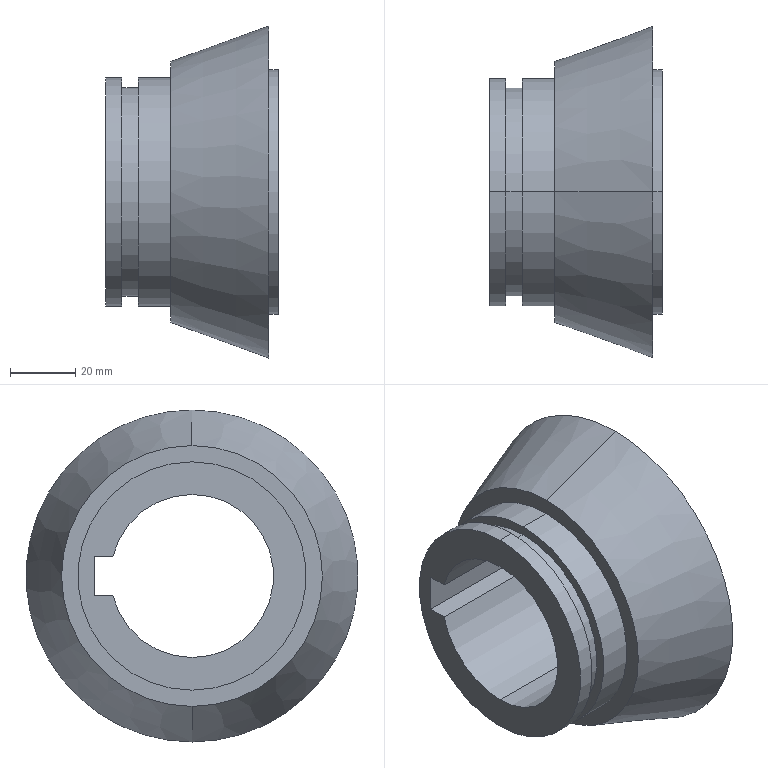Part | SolidWorks | features ICE 2, Revolution 1 | 1 solid | 25 faces | box 53 x 101.838 x 101.838 mm | volume 175302 mm3 | cylinder 13 | plane 10 | cone 2 | commonest cylinder face diameters 70 x4 50 x3 3 x2 64 x2 75 x2
STEP:
#1=CARTESIAN_POINT('',(43.,-32.5,1.5));
#2=VERTEX_POINT('',#1);
#3=CARTESIAN_POINT('',(43.,-32.5,-1.5));
#4=VERTEX_POINT('',#3);
#5=CARTESIAN_POINT('',(43.,-32.5,0.));
#6=DIRECTION('',(1.,0.,0.));
#7=DIRECTION('',(0.,0.,-1.));
#8=AXIS2_PLACEMENT_3D('',#5,#6,#7);
#9=CIRCLE('',#8,1.5);
#10=EDGE_CURVE('',#2,#4,#9,.T.);
#11=ORIENTED_EDGE('',*,*,#10,.F.);
#12=CARTESIAN_POINT('',(53.,-32.5,1.5));
#13=VERTEX_POINT('',#12);
#14=CARTESIAN_POINT('',(43.,-32.5,1.5));
#15=DIRECTION('',(1.,0.,0.));
#16=VECTOR('',#15,1000.);
#17=LINE('',#14,#16);
#18=EDGE_CURVE('',#2,#13,#17,.T.);
#19=ORIENTED_EDGE('',*,*,#18,.T.);
#20=CARTESIAN_POINT('',(53.,-32.5,-1.5));
#21=VERTEX_POINT('',#20);
#22=CARTESIAN_POINT('',(53.,-32.5,0.));
#23=DIRECTION('',(1.,0.,0.));
#24=DIRECTION('',(0.,0.,-1.));
#25=AXIS2_PLACEMENT_3D('',#22,#23,#24);
#26=CIRCLE('',#25,1.5);
#27=EDGE_CURVE('',#13,#21,#26,.T.);
#28=ORIENTED_EDGE('',*,*,#27,.T.);
#29=CARTESIAN_POINT('',(43.,-32.5,-1.5));
#30=DIRECTION('',(1.,0.,0.));
#31=VECTOR('',#30,1000.);
#32=LINE('',#29,#31);
#33=EDGE_CURVE('',#4,#21,#32,.T.);
#34=ORIENTED_EDGE('',*,*,#33,.F.);
#35=EDGE_LOOP('',(#11,#19,#28,#34));
#36=FACE_OUTER_BOUND('',#35,.T.);
#37=CARTESIAN_POINT('',(43.,-32.5,0.));
#38=DIRECTION('',(1.,0.,0.));
#39=DIRECTION('',(0.,0.,-1.));
#40=AXIS2_PLACEMENT_3D('',#37,#38,#39);
#41=CYLINDRICAL_SURFACE('',#40,1.5);
#42=ADVANCED_FACE('',(#36),#41,.F.);
#43=CARTESIAN_POINT('',(53.,0.,37.5));
#44=VERTEX_POINT('',#43);
#45=CARTESIAN_POINT('',(53.,0.,-37.5));
#46=VERTEX_POINT('',#45);
#47=CARTESIAN_POINT('',(53.,0.,0.));
#48=DIRECTION('',(-1.,0.,0.));
#49=DIRECTION('',(0.,0.,1.));
#50=AXIS2_PLACEMENT_3D('',#47,#48,#49);
#51=CIRCLE('',#50,37.5);
#52=EDGE_CURVE('',#44,#46,#51,.T.);
#53=ORIENTED_EDGE('',*,*,#52,.T.);
#54=CARTESIAN_POINT('',(50.,0.,-37.5));
#55=VERTEX_POINT('',#54);
#56=CARTESIAN_POINT('',(0.,0.,-37.5));
#57=DIRECTION('',(-1.,0.,0.));
#58=VECTOR('',#57,1000.);
#59=LINE('',#56,#58);
#60=EDGE_CURVE('',#46,#55,#59,.T.);
#61=ORIENTED_EDGE('',*,*,#60,.T.);
#62=CARTESIAN_POINT('',(50.,0.,37.5));
#63=VERTEX_POINT('',#62);
#64=CARTESIAN_POINT('',(50.,0.,0.));
#65=DIRECTION('',(-1.,0.,0.));
#66=DIRECTION('',(0.,0.,1.));
#67=AXIS2_PLACEMENT_3D('',#64,#65,#66);
#68=CIRCLE('',#67,37.5);
#69=EDGE_CURVE('',#63,#55,#68,.T.);
#70=ORIENTED_EDGE('',*,*,#69,.F.);
#71=CARTESIAN_POINT('',(0.,0.,37.5));
#72=DIRECTION('',(-1.,0.,0.));
#73=VECTOR('',#72,1000.);
#74=LINE('',#71,#73);
#75=EDGE_CURVE('',#44,#63,#74,.T.);
#76=ORIENTED_EDGE('',*,*,#75,.F.);
#77=EDGE_LOOP('',(#53,#61,#70,#76));
#78=FACE_OUTER_BOUND('',#77,.T.);
#79=CARTESIAN_POINT('',(0.,0.,0.));
#80=DIRECTION('',(-1.,0.,0.));
#81=DIRECTION('',(0.,0.,1.));
#82=AXIS2_PLACEMENT_3D('',#79,#80,#81);
#83=CYLINDRICAL_SURFACE('',#82,37.5);
#84=ADVANCED_FACE('',(#78),#83,.T.);
#85=CARTESIAN_POINT('',(20.,0.,40.));
#86=VERTEX_POINT('',#85);
#87=CARTESIAN_POINT('',(20.,0.,-40.));
#88=VERTEX_POINT('',#87);
#89=CARTESIAN_POINT('',(20.,0.,0.));
#90=DIRECTION('',(-1.,0.,0.));
#91=DIRECTION('',(0.,0.,1.));
#92=AXIS2_PLACEMENT_3D('',#89,#90,#91);
#93=CIRCLE('',#92,40.);
#94=EDGE_CURVE('',#86,#88,#93,.T.);
#95=ORIENTED_EDGE('',*,*,#94,.F.);
#96=CARTESIAN_POINT('',(50.,0.,50.919));
#97=VERTEX_POINT('',#96);
#98=CARTESIAN_POINT('',(50.,0.,50.919));
#99=DIRECTION('',(0.9397,0.,0.342));
#100=VECTOR('',#99,1000.);
#101=LINE('',#98,#100);
#102=EDGE_CURVE('',#86,#97,#101,.T.);
#103=ORIENTED_EDGE('',*,*,#102,.T.);
#104=CARTESIAN_POINT('',(50.,0.,-50.919));
#105=VERTEX_POINT('',#104);
#106=CARTESIAN_POINT('',(50.,0.,0.));
#107=DIRECTION('',(-1.,0.,0.));
#108=DIRECTION('',(0.,0.,1.));
#109=AXIS2_PLACEMENT_3D('',#106,#107,#108);
#110=CIRCLE('',#109,50.919);
#111=EDGE_CURVE('',#97,#105,#110,.T.);
#112=ORIENTED_EDGE('',*,*,#111,.T.);
#113=CARTESIAN_POINT('',(50.,0.,-50.919));
#114=DIRECTION('',(0.9397,0.,-0.342));
#115=VECTOR('',#114,1000.);
#116=LINE('',#113,#115);
#117=EDGE_CURVE('',#88,#105,#116,.T.);
#118=ORIENTED_EDGE('',*,*,#117,.F.);
#119=EDGE_LOOP('',(#95,#103,#112,#118));
#120=FACE_OUTER_BOUND('',#119,.T.);
#121=CARTESIAN_POINT('',(50.,0.,0.));
#122=DIRECTION('',(1.,0.,0.));
#123=DIRECTION('',(0.,0.,-1.));
#124=AXIS2_PLACEMENT_3D('',#121,#122,#123);
#125=CONICAL_SURFACE('',#124,50.919,0.3491);
#126=ADVANCED_FACE('',(#120),#125,.T.);
#127=CARTESIAN_POINT('',(20.,0.,35.));
#128=VERTEX_POINT('',#127);
#129=CARTESIAN_POINT('',(20.,0.,-35.));
#130=VERTEX_POINT('',#129);
#131=CARTESIAN_POINT('',(20.,0.,0.));
#132=DIRECTION('',(-1.,0.,0.));
#133=DIRECTION('',(0.,0.,1.));
#134=AXIS2_PLACEMENT_3D('',#131,#132,#133);
#135=CIRCLE('',#134,35.);
#136=EDGE_CURVE('',#128,#130,#135,.T.);
#137=ORIENTED_EDGE('',*,*,#136,.T.);
#138=CARTESIAN_POINT('',(10.,0.,-35.));
#139=VERTEX_POINT('',#138);
#140=CARTESIAN_POINT('',(0.,0.,-35.));
#141=DIRECTION('',(-1.,0.,0.));
#142=VECTOR('',#141,1000.);
#143=LINE('',#140,#142);
#144=EDGE_CURVE('',#130,#139,#143,.T.);
#145=ORIENTED_EDGE('',*,*,#144,.T.);
#146=CARTESIAN_POINT('',(10.,0.,35.));
#147=VERTEX_POINT('',#146);
#148=CARTESIAN_POINT('',(10.,0.,0.));
#149=DIRECTION('',(-1.,0.,0.));
#150=DIRECTION('',(0.,0.,1.));
#151=AXIS2_PLACEMENT_3D('',#148,#149,#150);
#152=CIRCLE('',#151,35.);
#153=EDGE_CURVE('',#147,#139,#152,.T.);
#154=ORIENTED_EDGE('',*,*,#153,.F.);
#155=CARTESIAN_POINT('',(0.,0.,35.));
#156=DIRECTION('',(-1.,0.,0.));
#157=VECTOR('',#156,1000.);
#158=LINE('',#155,#157);
#159=EDGE_CURVE('',#128,#147,#158,.T.);
#160=ORIENTED_EDGE('',*,*,#159,.F.);
#161=EDGE_LOOP('',(#137,#145,#154,#160));
#162=FACE_OUTER_BOUND('',#161,.T.);
#163=CARTESIAN_POINT('',(0.,0.,0.));
#164=DIRECTION('',(-1.,0.,0.));
#165=DIRECTION('',(0.,0.,1.));
#166=AXIS2_PLACEMENT_3D('',#163,#164,#165);
#167=CYLINDRICAL_SURFACE('',#166,35.);
#168=ADVANCED_FACE('',(#162),#167,.T.);
#169=CARTESIAN_POINT('',(10.,0.,32.));
#170=VERTEX_POINT('',#169);
#171=CARTESIAN_POINT('',(10.,0.,-32.));
#172=VERTEX_POINT('',#171);
#173=CARTESIAN_POINT('',(10.,0.,0.));
#174=DIRECTION('',(-1.,0.,0.));
#175=DIRECTION('',(0.,0.,1.));
#176=AXIS2_PLACEMENT_3D('',#173,#174,#175);
#177=CIRCLE('',#176,32.);
#178=EDGE_CURVE('',#170,#172,#177,.T.);
#179=ORIENTED_EDGE('',*,*,#178,.T.);
#180=CARTESIAN_POINT('',(5.,0.,-32.));
#181=VERTEX_POINT('',#180);
#182=CARTESIAN_POINT('',(0.,0.,-32.));
#183=DIRECTION('',(-1.,0.,0.));
#184=VECTOR('',#183,1000.);
#185=LINE('',#182,#184);
#186=EDGE_CURVE('',#172,#181,#185,.T.);
#187=ORIENTED_EDGE('',*,*,#186,.T.);
#188=CARTESIAN_POINT('',(5.,0.,32.));
#189=VERTEX_POINT('',#188);
#190=CARTESIAN_POINT('',(5.,0.,0.));
#191=DIRECTION('',(-1.,0.,0.));
#192=DIRECTION('',(0.,0.,1.));
#193=AXIS2_PLACEMENT_3D('',#190,#191,#192);
#194=CIRCLE('',#193,32.);
#195=EDGE_CURVE('',#189,#181,#194,.T.);
#196=ORIENTED_EDGE('',*,*,#195,.F.);
#197=CARTESIAN_POINT('',(0.,0.,32.));
#198=DIRECTION('',(-1.,0.,0.));
#199=VECTOR('',#198,1000.);
#200=LINE('',#197,#199);
#201=EDGE_CURVE('',#170,#189,#200,.T.);
#202=ORIENTED_EDGE('',*,*,#201,.F.);
#203=EDGE_LOOP('',(#179,#187,#196,#202));
#204=FACE_OUTER_BOUND('',#203,.T.);
#205=CARTESIAN_POINT('',(0.,0.,0.));
#206=DIRECTION('',(-1.,0.,0.));
#207=DIRECTION('',(0.,0.,1.));
#208=AXIS2_PLACEMENT_3D('',#205,#206,#207);
#209=CYLINDRICAL_SURFACE('',#208,32.);
#210=ADVANCED_FACE('',(#204),#209,.T.);
#211=CARTESIAN_POINT('',(5.,0.,35.));
#212=VERTEX_POINT('',#211);
#213=CARTESIAN_POINT('',(5.,0.,-35.));
#214=VERTEX_POINT('',#213);
#215=CARTESIAN_POINT('',(5.,0.,0.));
#216=DIRECTION('',(-1.,0.,0.));
#217=DIRECTION('',(0.,0.,1.));
#218=AXIS2_PLACEMENT_3D('',#215,#216,#217);
#219=CIRCLE('',#218,35.);
#220=EDGE_CURVE('',#212,#214,#219,.T.);
#221=ORIENTED_EDGE('',*,*,#220,.T.);
#222=CARTESIAN_POINT('',(0.,0.,-35.));
#223=VERTEX_POINT('',#222);
#224=CARTESIAN_POINT('',(0.,0.,-35.));
#225=DIRECTION('',(-1.,0.,0.));
#226=VECTOR('',#225,1000.);
#227=LINE('',#224,#226);
#228=EDGE_CURVE('',#214,#223,#227,.T.);
#229=ORIENTED_EDGE('',*,*,#228,.T.);
#230=CARTESIAN_POINT('',(0.,0.,35.));
#231=VERTEX_POINT('',#230);
#232=CARTESIAN_POINT('',(0.,0.,0.));
#233=DIRECTION('',(-1.,0.,0.));
#234=DIRECTION('',(0.,0.,1.));
#235=AXIS2_PLACEMENT_3D('',#232,#233,#234);
#236=CIRCLE('',#235,35.);
#237=EDGE_CURVE('',#231,#223,#236,.T.);
#238=ORIENTED_EDGE('',*,*,#237,.F.);
#239=CARTESIAN_POINT('',(0.,0.,35.));
#240=DIRECTION('',(-1.,0.,0.));
#241=VECTOR('',#240,1000.);
#242=LINE('',#239,#241);
#243=EDGE_CURVE('',#212,#231,#242,.T.);
#244=ORIENTED_EDGE('',*,*,#243,.F.);
#245=EDGE_LOOP('',(#221,#229,#238,#244));
#246=FACE_OUTER_BOUND('',#245,.T.);
#247=CARTESIAN_POINT('',(0.,0.,0.));
#248=DIRECTION('',(-1.,0.,0.));
#249=DIRECTION('',(0.,0.,1.));
#250=AXIS2_PLACEMENT_3D('',#247,#248,#249);
#251=CYLINDRICAL_SURFACE('',#250,35.);
#252=ADVANCED_FACE('',(#246),#251,.T.);
#253=CARTESIAN_POINT('',(53.,0.,-25.));
#254=VERTEX_POINT('',#253);
#255=CARTESIAN_POINT('',(53.,0.,25.));
#256=VERTEX_POINT('',#255);
#257=CARTESIAN_POINT('',(53.,0.,0.));
#258=DIRECTION('',(-1.,0.,0.));
#259=DIRECTION('',(0.,0.,1.));
#260=AXIS2_PLACEMENT_3D('',#257,#258,#259);
#261=CIRCLE('',#260,25.);
#262=EDGE_CURVE('',#254,#256,#261,.T.);
#263=ORIENTED_EDGE('',*,*,#262,.F.);
#264=CARTESIAN_POINT('',(0.,0.,-25.));
#265=VERTEX_POINT('',#264);
#266=CARTESIAN_POINT('',(0.,0.,-25.));
#267=DIRECTION('',(-1.,0.,0.));
#268=VECTOR('',#267,1000.);
#269=LINE('',#266,#268);
#270=EDGE_CURVE('',#254,#265,#269,.T.);
#271=ORIENTED_EDGE('',*,*,#270,.T.);
#272=CARTESIAN_POINT('',(0.,0.,25.));
#273=VERTEX_POINT('',#272);
#274=CARTESIAN_POINT('',(0.,0.,0.));
#275=DIRECTION('',(-1.,0.,0.));
#276=DIRECTION('',(0.,0.,1.));
#277=AXIS2_PLACEMENT_3D('',#274,#275,#276);
#278=CIRCLE('',#277,25.);
#279=EDGE_CURVE('',#265,#273,#278,.T.);
#280=ORIENTED_EDGE('',*,*,#279,.T.);
#281=CARTESIAN_POINT('',(0.,0.,25.));
#282=DIRECTION('',(-1.,0.,0.));
#283=VECTOR('',#282,1000.);
#284=LINE('',#281,#283);
#285=EDGE_CURVE('',#256,#273,#284,.T.);
#286=ORIENTED_EDGE('',*,*,#285,.F.);
#287=EDGE_LOOP('',(#263,#271,#280,#286));
#288=FACE_OUTER_BOUND('',#287,.T.);
#289=CARTESIAN_POINT('',(0.,0.,0.));
#290=DIRECTION('',(-1.,0.,0.));
#291=DIRECTION('',(0.,0.,1.));
#292=AXIS2_PLACEMENT_3D('',#289,#290,#291);
#293=CYLINDRICAL_SURFACE('',#292,25.);
#294=ADVANCED_FACE('',(#288),#293,.F.);
#295=CARTESIAN_POINT('',(53.,24.269,6.));
#296=VERTEX_POINT('',#295);
#297=CARTESIAN_POINT('',(53.,0.,0.));
#298=DIRECTION('',(-1.,0.,0.));
#299=DIRECTION('',(0.,0.,1.));
#300=AXIS2_PLACEMENT_3D('',#297,#298,#299);
#301=CIRCLE('',#300,25.);
#302=EDGE_CURVE('',#256,#296,#301,.T.);
#303=ORIENTED_EDGE('',*,*,#302,.F.);
#304=ORIENTED_EDGE('',*,*,#285,.T.);
#305=CARTESIAN_POINT('',(0.,24.269,6.));
#306=VERTEX_POINT('',#305);
#307=CARTESIAN_POINT('',(0.,0.,0.));
#308=DIRECTION('',(-1.,0.,0.));
#309=DIRECTION('',(0.,0.,1.));
#310=AXIS2_PLACEMENT_3D('',#307,#308,#309);
#311=CIRCLE('',#310,25.);
#312=EDGE_CURVE('',#273,#306,#311,.T.);
#313=ORIENTED_EDGE('',*,*,#312,.T.);
#314=CARTESIAN_POINT('',(0.,24.269,6.));
#315=DIRECTION('',(1.,0.,0.));
#316=VECTOR('',#315,1000.);
#317=LINE('',#314,#316);
#318=EDGE_CURVE('',#306,#296,#317,.T.);
#319=ORIENTED_EDGE('',*,*,#318,.T.);
#320=EDGE_LOOP('',(#303,#304,#313,#319));
#321=FACE_OUTER_BOUND('',#320,.T.);
#322=CARTESIAN_POINT('',(0.,0.,0.));
#323=DIRECTION('',(-1.,0.,0.));
#324=DIRECTION('',(0.,0.,1.));
#325=AXIS2_PLACEMENT_3D('',#322,#323,#324);
#326=CYLINDRICAL_SURFACE('',#325,25.);
#327=ADVANCED_FACE('',(#321),#326,.F.);
#328=ORIENTED_EDGE('',*,*,#270,.F.);
#329=CARTESIAN_POINT('',(53.,24.269,-6.));
#330=VERTEX_POINT('',#329);
#331=CARTESIAN_POINT('',(53.,0.,0.));
#332=DIRECTION('',(-1.,0.,0.));
#333=DIRECTION('',(0.,0.,1.));
#334=AXIS2_PLACEMENT_3D('',#331,#332,#333);
#335=CIRCLE('',#334,25.);
#336=EDGE_CURVE('',#330,#254,#335,.T.);
#337=ORIENTED_EDGE('',*,*,#336,.F.);
#338=CARTESIAN_POINT('',(0.,24.269,-6.));
#339=VERTEX_POINT('',#338);
#340=CARTESIAN_POINT('',(0.,24.269,-6.));
#341=DIRECTION('',(-1.,0.,0.));
#342=VECTOR('',#341,1000.);
#343=LINE('',#340,#342);
#344=EDGE_CURVE('',#330,#339,#343,.T.);
#345=ORIENTED_EDGE('',*,*,#344,.T.);
#346=CARTESIAN_POINT('',(0.,0.,0.));
#347=DIRECTION('',(-1.,0.,0.));
#348=DIRECTION('',(0.,0.,1.));
#349=AXIS2_PLACEMENT_3D('',#346,#347,#348);
#350=CIRCLE('',#349,25.);
#351=EDGE_CURVE('',#339,#265,#350,.T.);
#352=ORIENTED_EDGE('',*,*,#351,.T.);
#353=EDGE_LOOP('',(#328,#337,#345,#352));
#354=FACE_OUTER_BOUND('',#353,.T.);
#355=CARTESIAN_POINT('',(0.,0.,0.));
#356=DIRECTION('',(-1.,0.,0.));
#357=DIRECTION('',(0.,0.,1.));
#358=AXIS2_PLACEMENT_3D('',#355,#356,#357);
#359=CYLINDRICAL_SURFACE('',#358,25.);
#360=ADVANCED_FACE('',(#354),#359,.F.);
#361=ORIENTED_EDGE('',*,*,#351,.F.);
#362=CARTESIAN_POINT('',(0.,30.,-6.));
#363=VERTEX_POINT('',#362);
#364=CARTESIAN_POINT('',(0.,30.,-6.));
#365=DIRECTION('',(0.,1.,0.));
#366=VECTOR('',#365,1000.);
#367=LINE('',#364,#366);
#368=EDGE_CURVE('',#339,#363,#367,.T.);
#369=ORIENTED_EDGE('',*,*,#368,.T.);
#370=CARTESIAN_POINT('',(0.,30.,6.));
#371=VERTEX_POINT('',#370);
#372=CARTESIAN_POINT('',(0.,30.,6.));
#373=DIRECTION('',(0.,0.,1.));
#374=VECTOR('',#373,1000.);
#375=LINE('',#372,#374);
#376=EDGE_CURVE('',#363,#371,#375,.T.);
#377=ORIENTED_EDGE('',*,*,#376,.T.);
#378=CARTESIAN_POINT('',(0.,30.,6.));
#379=DIRECTION('',(0.,-1.,0.));
#380=VECTOR('',#379,1000.);
#381=LINE('',#378,#380);
#382=EDGE_CURVE('',#371,#306,#381,.T.);
#383=ORIENTED_EDGE('',*,*,#382,.T.);
#384=ORIENTED_EDGE('',*,*,#312,.F.);
#385=ORIENTED_EDGE('',*,*,#279,.F.);
#386=EDGE_LOOP('',(#361,#369,#377,#383,#384,#385));
#387=FACE_BOUND('',#386,.T.);
#388=ORIENTED_EDGE('',*,*,#237,.T.);
#389=CARTESIAN_POINT('',(0.,0.,0.));
#390=DIRECTION('',(-1.,0.,0.));
#391=DIRECTION('',(0.,0.,1.));
#392=AXIS2_PLACEMENT_3D('',#389,#390,#391);
#393=CIRCLE('',#392,35.);
#394=EDGE_CURVE('',#223,#231,#393,.T.);
#395=ORIENTED_EDGE('',*,*,#394,.T.);
#396=EDGE_LOOP('',(#388,#395));
#397=FACE_OUTER_BOUND('',#396,.T.);
#398=CARTESIAN_POINT('',(0.,25.,0.));
#399=DIRECTION('',(1.,0.,0.));
#400=DIRECTION('',(0.,0.,-1.));
#401=AXIS2_PLACEMENT_3D('',#398,#399,#400);
#402=PLANE('',#401);
#403=ADVANCED_FACE('',(#387,#397),#402,.F.);
#404=ORIENTED_EDGE('',*,*,#228,.F.);
#405=CARTESIAN_POINT('',(5.,0.,0.));
#406=DIRECTION('',(-1.,0.,0.));
#407=DIRECTION('',(0.,0.,1.));
#408=AXIS2_PLACEMENT_3D('',#405,#406,#407);
#409=CIRCLE('',#408,35.);
#410=EDGE_CURVE('',#214,#212,#409,.T.);
#411=ORIENTED_EDGE('',*,*,#410,.T.);
#412=ORIENTED_EDGE('',*,*,#243,.T.);
#413=ORIENTED_EDGE('',*,*,#394,.F.);
#414=EDGE_LOOP('',(#404,#411,#412,#413));
#415=FACE_OUTER_BOUND('',#414,.T.);
#416=CARTESIAN_POINT('',(0.,0.,0.));
#417=DIRECTION('',(-1.,0.,0.));
#418=DIRECTION('',(0.,0.,1.));
#419=AXIS2_PLACEMENT_3D('',#416,#417,#418);
#420=CYLINDRICAL_SURFACE('',#419,35.);
#421=ADVANCED_FACE('',(#415),#420,.T.);
#422=ORIENTED_EDGE('',*,*,#220,.F.);
#423=ORIENTED_EDGE('',*,*,#410,.F.);
#424=EDGE_LOOP('',(#422,#423));
#425=FACE_OUTER_BOUND('',#424,.T.);
#426=ORIENTED_EDGE('',*,*,#195,.T.);
#427=CARTESIAN_POINT('',(5.,0.,0.));
#428=DIRECTION('',(-1.,0.,0.));
#429=DIRECTION('',(0.,0.,1.));
#430=AXIS2_PLACEMENT_3D('',#427,#428,#429);
#431=CIRCLE('',#430,32.);
#432=EDGE_CURVE('',#181,#189,#431,.T.);
#433=ORIENTED_EDGE('',*,*,#432,.T.);
#434=EDGE_LOOP('',(#426,#433));
#435=FACE_BOUND('',#434,.T.);
#436=CARTESIAN_POINT('',(5.,35.,0.));
#437=DIRECTION('',(-1.,0.,0.));
#438=DIRECTION('',(0.,0.,1.));
#439=AXIS2_PLACEMENT_3D('',#436,#437,#438);
#440=PLANE('',#439);
#441=ADVANCED_FACE('',(#425,#435),#440,.F.);
#442=ORIENTED_EDGE('',*,*,#186,.F.);
#443=CARTESIAN_POINT('',(10.,0.,0.));
#444=DIRECTION('',(-1.,0.,0.));
#445=DIRECTION('',(0.,0.,1.));
#446=AXIS2_PLACEMENT_3D('',#443,#444,#445);
#447=CIRCLE('',#446,32.);
#448=EDGE_CURVE('',#172,#170,#447,.T.);
#449=ORIENTED_EDGE('',*,*,#448,.T.);
#450=ORIENTED_EDGE('',*,*,#201,.T.);
#451=ORIENTED_EDGE('',*,*,#432,.F.);
#452=EDGE_LOOP('',(#442,#449,#450,#451));
#453=FACE_OUTER_BOUND('',#452,.T.);
#454=CARTESIAN_POINT('',(0.,0.,0.));
#455=DIRECTION('',(-1.,0.,0.));
#456=DIRECTION('',(0.,0.,1.));
#457=AXIS2_PLACEMENT_3D('',#454,#455,#456);
#458=CYLINDRICAL_SURFACE('',#457,32.);
#459=ADVANCED_FACE('',(#453),#458,.T.);
#460=ORIENTED_EDGE('',*,*,#178,.F.);
#461=ORIENTED_EDGE('',*,*,#448,.F.);
#462=EDGE_LOOP('',(#460,#461));
#463=FACE_BOUND('',#462,.T.);
#464=ORIENTED_EDGE('',*,*,#153,.T.);
#465=CARTESIAN_POINT('',(10.,0.,0.));
#466=DIRECTION('',(-1.,0.,0.));
#467=DIRECTION('',(0.,0.,1.));
#468=AXIS2_PLACEMENT_3D('',#465,#466,#467);
#469=CIRCLE('',#468,35.);
#470=EDGE_CURVE('',#139,#147,#469,.T.);
#471=ORIENTED_EDGE('',*,*,#470,.T.);
#472=EDGE_LOOP('',(#464,#471));
#473=FACE_OUTER_BOUND('',#472,.T.);
#474=CARTESIAN_POINT('',(10.,32.,0.));
#475=DIRECTION('',(1.,0.,0.));
#476=DIRECTION('',(0.,0.,-1.));
#477=AXIS2_PLACEMENT_3D('',#474,#475,#476);
#478=PLANE('',#477);
#479=ADVANCED_FACE('',(#463,#473),#478,.F.);
#480=ORIENTED_EDGE('',*,*,#144,.F.);
#481=CARTESIAN_POINT('',(20.,0.,0.));
#482=DIRECTION('',(-1.,0.,0.));
#483=DIRECTION('',(0.,0.,1.));
#484=AXIS2_PLACEMENT_3D('',#481,#482,#483);
#485=CIRCLE('',#484,35.);
#486=EDGE_CURVE('',#130,#128,#485,.T.);
#487=ORIENTED_EDGE('',*,*,#486,.T.);
#488=ORIENTED_EDGE('',*,*,#159,.T.);
#489=ORIENTED_EDGE('',*,*,#470,.F.);
#490=EDGE_LOOP('',(#480,#487,#488,#489));
#491=FACE_OUTER_BOUND('',#490,.T.);
#492=CARTESIAN_POINT('',(0.,0.,0.));
#493=DIRECTION('',(-1.,0.,0.));
#494=DIRECTION('',(0.,0.,1.));
#495=AXIS2_PLACEMENT_3D('',#492,#493,#494);
#496=CYLINDRICAL_SURFACE('',#495,35.);
#497=ADVANCED_FACE('',(#491),#496,.T.);
#498=ORIENTED_EDGE('',*,*,#136,.F.);
#499=ORIENTED_EDGE('',*,*,#486,.F.);
#500=EDGE_LOOP('',(#498,#499));
#501=FACE_BOUND('',#500,.T.);
#502=CARTESIAN_POINT('',(20.,0.,0.));
#503=DIRECTION('',(-1.,0.,0.));
#504=DIRECTION('',(0.,0.,1.));
#505=AXIS2_PLACEMENT_3D('',#502,#503,#504);
#506=CIRCLE('',#505,40.);
#507=EDGE_CURVE('',#88,#86,#506,.T.);
#508=ORIENTED_EDGE('',*,*,#507,.T.);
#509=ORIENTED_EDGE('',*,*,#94,.T.);
#510=EDGE_LOOP('',(#508,#509));
#511=FACE_OUTER_BOUND('',#510,.T.);
#512=CARTESIAN_POINT('',(20.,35.,0.));
#513=DIRECTION('',(1.,0.,0.));
#514=DIRECTION('',(0.,0.,-1.));
#515=AXIS2_PLACEMENT_3D('',#512,#513,#514);
#516=PLANE('',#515);
#517=ADVANCED_FACE('',(#501,#511),#516,.F.);
#518=ORIENTED_EDGE('',*,*,#102,.F.);
#519=ORIENTED_EDGE('',*,*,#507,.F.);
#520=ORIENTED_EDGE('',*,*,#117,.T.);
#521=CARTESIAN_POINT('',(50.,0.,0.));
#522=DIRECTION('',(-1.,0.,0.));
#523=DIRECTION('',(0.,0.,1.));
#524=AXIS2_PLACEMENT_3D('',#521,#522,#523);
#525=CIRCLE('',#524,50.919);
#526=EDGE_CURVE('',#105,#97,#525,.T.);
#527=ORIENTED_EDGE('',*,*,#526,.T.);
#528=EDGE_LOOP('',(#518,#519,#520,#527));
#529=FACE_OUTER_BOUND('',#528,.T.);
#530=CARTESIAN_POINT('',(50.,0.,0.));
#531=DIRECTION('',(1.,0.,0.));
#532=DIRECTION('',(0.,0.,-1.));
#533=AXIS2_PLACEMENT_3D('',#530,#531,#532);
#534=CONICAL_SURFACE('',#533,50.919,0.3491);
#535=ADVANCED_FACE('',(#529),#534,.T.);
#536=ORIENTED_EDGE('',*,*,#526,.F.);
#537=ORIENTED_EDGE('',*,*,#111,.F.);
#538=EDGE_LOOP('',(#536,#537));
#539=FACE_OUTER_BOUND('',#538,.T.);
#540=ORIENTED_EDGE('',*,*,#69,.T.);
#541=CARTESIAN_POINT('',(50.,0.,0.));
#542=DIRECTION('',(-1.,0.,0.));
#543=DIRECTION('',(0.,0.,1.));
#544=AXIS2_PLACEMENT_3D('',#541,#542,#543);
#545=CIRCLE('',#544,37.5);
#546=EDGE_CURVE('',#55,#63,#545,.T.);
#547=ORIENTED_EDGE('',*,*,#546,.T.);
#548=EDGE_LOOP('',(#540,#547));
#549=FACE_BOUND('',#548,.T.);
#550=CARTESIAN_POINT('',(50.,50.919,0.));
#551=DIRECTION('',(-1.,0.,0.));
#552=DIRECTION('',(0.,0.,1.));
#553=AXIS2_PLACEMENT_3D('',#550,#551,#552);
#554=PLANE('',#553);
#555=ADVANCED_FACE('',(#539,#549),#554,.F.);
#556=ORIENTED_EDGE('',*,*,#60,.F.);
#557=CARTESIAN_POINT('',(53.,0.,0.));
#558=DIRECTION('',(-1.,0.,0.));
#559=DIRECTION('',(0.,0.,1.));
#560=AXIS2_PLACEMENT_3D('',#557,#558,#559);
#561=CIRCLE('',#560,37.5);
#562=EDGE_CURVE('',#46,#44,#561,.T.);
#563=ORIENTED_EDGE('',*,*,#562,.T.);
#564=ORIENTED_EDGE('',*,*,#75,.T.);
#565=ORIENTED_EDGE('',*,*,#546,.F.);
#566=EDGE_LOOP('',(#556,#563,#564,#565));
#567=FACE_OUTER_BOUND('',#566,.T.);
#568=CARTESIAN_POINT('',(0.,0.,0.));
#569=DIRECTION('',(-1.,0.,0.));
#570=DIRECTION('',(0.,0.,1.));
#571=AXIS2_PLACEMENT_3D('',#568,#569,#570);
#572=CYLINDRICAL_SURFACE('',#571,37.5);
#573=ADVANCED_FACE('',(#567),#572,.T.);
#574=CARTESIAN_POINT('',(53.,-32.5,0.));
#575=DIRECTION('',(1.,0.,0.));
#576=DIRECTION('',(0.,0.,-1.));
#577=AXIS2_PLACEMENT_3D('',#574,#575,#576);
#578=CIRCLE('',#577,1.5);
#579=EDGE_CURVE('',#21,#13,#578,.T.);
#580=ORIENTED_EDGE('',*,*,#579,.F.);
#581=ORIENTED_EDGE('',*,*,#27,.F.);
#582=EDGE_LOOP('',(#580,#581));
#583=FACE_BOUND('',#582,.T.);
#584=ORIENTED_EDGE('',*,*,#52,.F.);
#585=ORIENTED_EDGE('',*,*,#562,.F.);
#586=EDGE_LOOP('',(#584,#585));
#587=FACE_OUTER_BOUND('',#586,.T.);
#588=CARTESIAN_POINT('',(53.,30.,-6.));
#589=VERTEX_POINT('',#588);
#590=CARTESIAN_POINT('',(53.,30.,6.));
#591=VERTEX_POINT('',#590);
#592=CARTESIAN_POINT('',(53.,30.,6.));
#593=DIRECTION('',(0.,0.,1.));
#594=VECTOR('',#593,1000.);
#595=LINE('',#592,#594);
#596=EDGE_CURVE('',#589,#591,#595,.T.);
#597=ORIENTED_EDGE('',*,*,#596,.F.);
#598=CARTESIAN_POINT('',(53.,37.5,-6.));
#599=DIRECTION('',(0.,-1.,0.));
#600=VECTOR('',#599,1000.);
#601=LINE('',#598,#600);
#602=EDGE_CURVE('',#589,#330,#601,.T.);
#603=ORIENTED_EDGE('',*,*,#602,.T.);
#604=ORIENTED_EDGE('',*,*,#336,.T.);
#605=ORIENTED_EDGE('',*,*,#262,.T.);
#606=ORIENTED_EDGE('',*,*,#302,.T.);
#607=CARTESIAN_POINT('',(53.,30.,6.));
#608=DIRECTION('',(0.,-1.,0.));
#609=VECTOR('',#608,1000.);
#610=LINE('',#607,#609);
#611=EDGE_CURVE('',#591,#296,#610,.T.);
#612=ORIENTED_EDGE('',*,*,#611,.F.);
#613=EDGE_LOOP('',(#597,#603,#604,#605,#606,#612));
#614=FACE_BOUND('',#613,.T.);
#615=CARTESIAN_POINT('',(53.,37.5,0.));
#616=DIRECTION('',(-1.,0.,0.));
#617=DIRECTION('',(0.,0.,1.));
#618=AXIS2_PLACEMENT_3D('',#615,#616,#617);
#619=PLANE('',#618);
#620=ADVANCED_FACE('',(#583,#587,#614),#619,.F.);
#621=ORIENTED_EDGE('',*,*,#602,.F.);
#622=CARTESIAN_POINT('',(0.,30.,-6.));
#623=DIRECTION('',(1.,0.,0.));
#624=VECTOR('',#623,1000.);
#625=LINE('',#622,#624);
#626=EDGE_CURVE('',#363,#589,#625,.T.);
#627=ORIENTED_EDGE('',*,*,#626,.F.);
#628=ORIENTED_EDGE('',*,*,#368,.F.);
#629=ORIENTED_EDGE('',*,*,#344,.F.);
#630=EDGE_LOOP('',(#621,#627,#628,#629));
#631=FACE_OUTER_BOUND('',#630,.T.);
#632=CARTESIAN_POINT('',(0.,30.,-6.));
#633=DIRECTION('',(0.,0.,-1.));
#634=DIRECTION('',(0.,1.,0.));
#635=AXIS2_PLACEMENT_3D('',#632,#633,#634);
#636=PLANE('',#635);
#637=ADVANCED_FACE('',(#631),#636,.F.);
#638=ORIENTED_EDGE('',*,*,#382,.F.);
#639=CARTESIAN_POINT('',(0.,30.,6.));
#640=DIRECTION('',(1.,0.,0.));
#641=VECTOR('',#640,1000.);
#642=LINE('',#639,#641);
#643=EDGE_CURVE('',#371,#591,#642,.T.);
#644=ORIENTED_EDGE('',*,*,#643,.T.);
#645=ORIENTED_EDGE('',*,*,#611,.T.);
#646=ORIENTED_EDGE('',*,*,#318,.F.);
#647=EDGE_LOOP('',(#638,#644,#645,#646));
#648=FACE_OUTER_BOUND('',#647,.T.);
#649=CARTESIAN_POINT('',(0.,30.,6.));
#650=DIRECTION('',(0.,0.,1.));
#651=DIRECTION('',(0.,-1.,0.));
#652=AXIS2_PLACEMENT_3D('',#649,#650,#651);
#653=PLANE('',#652);
#654=ADVANCED_FACE('',(#648),#653,.F.);
#655=ORIENTED_EDGE('',*,*,#596,.T.);
#656=ORIENTED_EDGE('',*,*,#643,.F.);
#657=ORIENTED_EDGE('',*,*,#376,.F.);
#658=ORIENTED_EDGE('',*,*,#626,.T.);
#659=EDGE_LOOP('',(#655,#656,#657,#658));
#660=FACE_OUTER_BOUND('',#659,.T.);
#661=CARTESIAN_POINT('',(0.,30.,6.));
#662=DIRECTION('',(0.,1.,0.));
#663=DIRECTION('',(0.,0.,1.));
#664=AXIS2_PLACEMENT_3D('',#661,#662,#663);
#665=PLANE('',#664);
#666=ADVANCED_FACE('',(#660),#665,.F.);
#667=ORIENTED_EDGE('',*,*,#18,.F.);
#668=CARTESIAN_POINT('',(43.,-32.5,0.));
#669=DIRECTION('',(1.,0.,0.));
#670=DIRECTION('',(0.,0.,-1.));
#671=AXIS2_PLACEMENT_3D('',#668,#669,#670);
#672=CIRCLE('',#671,1.5);
#673=EDGE_CURVE('',#4,#2,#672,.T.);
#674=ORIENTED_EDGE('',*,*,#673,.F.);
#675=ORIENTED_EDGE('',*,*,#33,.T.);
#676=ORIENTED_EDGE('',*,*,#579,.T.);
#677=EDGE_LOOP('',(#667,#674,#675,#676));
#678=FACE_OUTER_BOUND('',#677,.T.);
#679=CARTESIAN_POINT('',(43.,-32.5,0.));
#680=DIRECTION('',(1.,0.,0.));
#681=DIRECTION('',(0.,0.,-1.));
#682=AXIS2_PLACEMENT_3D('',#679,#680,#681);
#683=CYLINDRICAL_SURFACE('',#682,1.5);
#684=ADVANCED_FACE('',(#678),#683,.F.);
#685=ORIENTED_EDGE('',*,*,#673,.T.);
#686=ORIENTED_EDGE('',*,*,#10,.T.);
#687=EDGE_LOOP('',(#685,#686));
#688=FACE_OUTER_BOUND('',#687,.T.);
#689=CARTESIAN_POINT('',(43.,-32.5,0.));
#690=DIRECTION('',(1.,0.,0.));
#691=DIRECTION('',(0.,0.,-1.));
#692=AXIS2_PLACEMENT_3D('',#689,#690,#691);
#693=PLANE('',#692);
#694=ADVANCED_FACE('',(#688),#693,.T.);
#695=CLOSED_SHELL('',(#42,#84,#126,#168,#210,#252,#294,#327,#360,#403,#421,#441,#459,#479,#497,#517,#535,#555,#573,#620,#637,#654,#666,#684,#694));
#696=MANIFOLD_SOLID_BREP('',#695);
#697=CARTESIAN_POINT('',(0.,0.,0.));
#698=DIRECTION('',(0.,0.,1.));
#699=DIRECTION('',(1.,0.,0.));
#700=AXIS2_PLACEMENT_3D('',#697,#698,#699);
#701=(LENGTH_UNIT()NAMED_UNIT(*)SI_UNIT(.MILLI.,.METRE.));
#702=UNCERTAINTY_MEASURE_WITH_UNIT(LENGTH_MEASURE(0.00001),#701,'','');
#703=(NAMED_UNIT(*)PLANE_ANGLE_UNIT()SI_UNIT($,.RADIAN.));
#704=(NAMED_UNIT(*)SI_UNIT($,.STERADIAN.)SOLID_ANGLE_UNIT());
#705=(GEOMETRIC_REPRESENTATION_CONTEXT(3)GLOBAL_UNCERTAINTY_ASSIGNED_CONTEXT((#702))GLOBAL_UNIT_ASSIGNED_CONTEXT((#701,#703,#704))REPRESENTATION_CONTEXT('',''));
#706=ADVANCED_BREP_SHAPE_REPRESENTATION('',(#696,#700),#705);